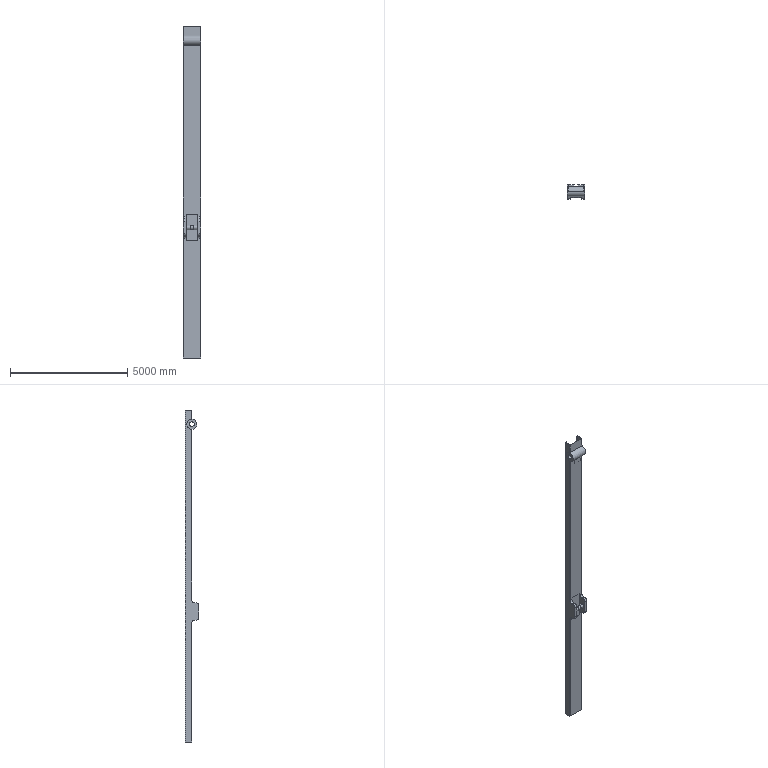Part | SolidWorks | features ICE 11, Fillet 2, Extrusion 1 | 1 solid | 64 faces | box 750 x 589 x 14150 mm | volume 669271540 mm3 | plane 42 | cylinder 22 | commonest cylinder face diameters 240 x8 180 x4 424.239 x4 110 x2 170 x2 200 x2